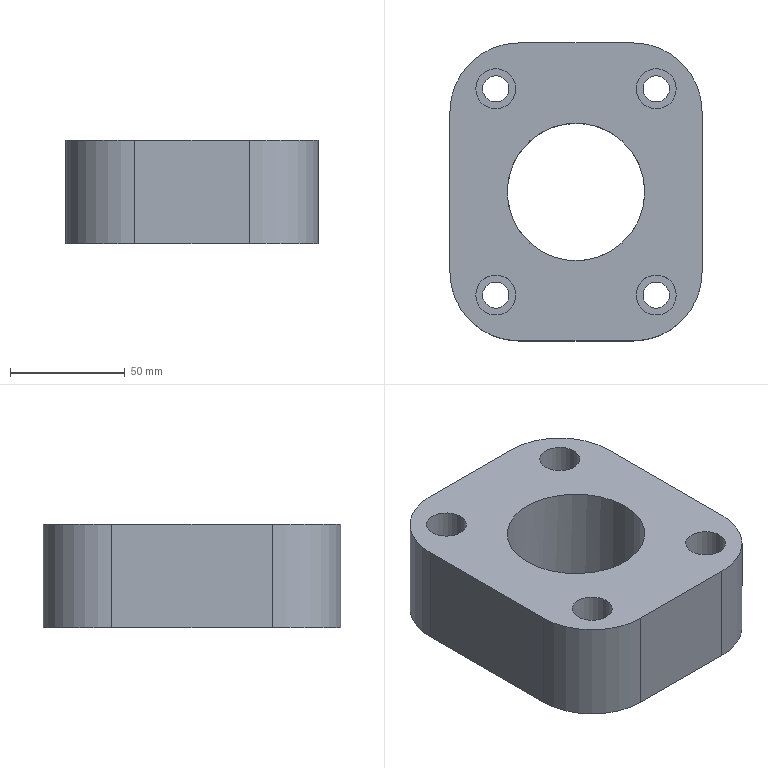Part | NX | features solid 2 | 1 solid | 23 faces | box 110 x 130 x 45 mm | volume 451871 mm3 | cylinder 13 | plane 10 | commonest cylinder face diameters 60 x5 11.5 x4 17.5 x4
STEP:
#1=CARTESIAN_POINT('',(-330.,55.,45.));
#2=VERTEX_POINT('',#1);
#3=CARTESIAN_POINT('',(-280.,55.,45.));
#4=VERTEX_POINT('',#3);
#5=CARTESIAN_POINT('',(-415.478,55.,45.));
#6=DIRECTION('',(-1.,0.,0.));
#7=VECTOR('',#6,1000.);
#8=LINE('',#5,#7);
#9=EDGE_CURVE('',#2,#4,#8,.F.);
#10=ORIENTED_EDGE('',*,*,#9,.T.);
#11=CARTESIAN_POINT('',(-250.,25.,45.));
#12=VERTEX_POINT('',#11);
#13=CARTESIAN_POINT('',(-280.,25.,45.));
#14=DIRECTION('',(0.,0.,1.));
#15=DIRECTION('',(1.,0.,0.));
#16=AXIS2_PLACEMENT_3D('',#13,#14,#15);
#17=CIRCLE('',#16,30.);
#18=EDGE_CURVE('',#4,#12,#17,.F.);
#19=ORIENTED_EDGE('',*,*,#18,.T.);
#20=CARTESIAN_POINT('',(-250.,-45.,45.));
#21=VERTEX_POINT('',#20);
#22=CARTESIAN_POINT('',(-250.,-10.,45.));
#23=DIRECTION('',(0.,-1.,0.));
#24=VECTOR('',#23,1000.);
#25=LINE('',#22,#24);
#26=EDGE_CURVE('',#21,#12,#25,.F.);
#27=ORIENTED_EDGE('',*,*,#26,.F.);
#28=CARTESIAN_POINT('',(-280.,-75.,45.));
#29=VERTEX_POINT('',#28);
#30=CARTESIAN_POINT('',(-280.,-45.,45.));
#31=DIRECTION('',(0.,0.,1.));
#32=DIRECTION('',(1.,0.,0.));
#33=AXIS2_PLACEMENT_3D('',#30,#31,#32);
#34=CIRCLE('',#33,30.);
#35=EDGE_CURVE('',#21,#29,#34,.F.);
#36=ORIENTED_EDGE('',*,*,#35,.T.);
#37=CARTESIAN_POINT('',(-330.,-75.,45.));
#38=VERTEX_POINT('',#37);
#39=CARTESIAN_POINT('',(-305.,-75.,45.));
#40=DIRECTION('',(-1.,0.,0.));
#41=VECTOR('',#40,1000.);
#42=LINE('',#39,#41);
#43=EDGE_CURVE('',#38,#29,#42,.F.);
#44=ORIENTED_EDGE('',*,*,#43,.F.);
#45=CARTESIAN_POINT('',(-360.,-45.,45.));
#46=VERTEX_POINT('',#45);
#47=CARTESIAN_POINT('',(-330.,-45.,45.));
#48=DIRECTION('',(0.,0.,1.));
#49=DIRECTION('',(1.,0.,0.));
#50=AXIS2_PLACEMENT_3D('',#47,#48,#49);
#51=CIRCLE('',#50,30.);
#52=EDGE_CURVE('',#38,#46,#51,.F.);
#53=ORIENTED_EDGE('',*,*,#52,.T.);
#54=CARTESIAN_POINT('',(-360.,25.,45.));
#55=VERTEX_POINT('',#54);
#56=CARTESIAN_POINT('',(-360.,-10.,45.));
#57=DIRECTION('',(0.,-1.,0.));
#58=VECTOR('',#57,1000.);
#59=LINE('',#56,#58);
#60=EDGE_CURVE('',#46,#55,#59,.F.);
#61=ORIENTED_EDGE('',*,*,#60,.T.);
#62=CARTESIAN_POINT('',(-330.,25.,45.));
#63=DIRECTION('',(0.,0.,1.));
#64=DIRECTION('',(1.,0.,0.));
#65=AXIS2_PLACEMENT_3D('',#62,#63,#64);
#66=CIRCLE('',#65,30.);
#67=EDGE_CURVE('',#55,#2,#66,.F.);
#68=ORIENTED_EDGE('',*,*,#67,.T.);
#69=EDGE_LOOP('',(#10,#19,#27,#36,#44,#53,#61,#68));
#70=FACE_BOUND('',#69,.T.);
#71=CARTESIAN_POINT('',(-334.25,35.,45.));
#72=VERTEX_POINT('',#71);
#73=CARTESIAN_POINT('',(-340.,35.,45.));
#74=DIRECTION('',(0.,0.,1.));
#75=DIRECTION('',(1.,0.,0.));
#76=AXIS2_PLACEMENT_3D('',#73,#74,#75);
#77=CIRCLE('',#76,5.75);
#78=EDGE_CURVE('',#72,#72,#77,.F.);
#79=ORIENTED_EDGE('',*,*,#78,.F.);
#80=EDGE_LOOP('',(#79));
#81=FACE_BOUND('',#80,.T.);
#82=CARTESIAN_POINT('',(-264.25,35.,45.));
#83=VERTEX_POINT('',#82);
#84=CARTESIAN_POINT('',(-270.,35.,45.));
#85=DIRECTION('',(0.,0.,1.));
#86=DIRECTION('',(1.,0.,0.));
#87=AXIS2_PLACEMENT_3D('',#84,#85,#86);
#88=CIRCLE('',#87,5.75);
#89=EDGE_CURVE('',#83,#83,#88,.F.);
#90=ORIENTED_EDGE('',*,*,#89,.F.);
#91=EDGE_LOOP('',(#90));
#92=FACE_BOUND('',#91,.T.);
#93=CARTESIAN_POINT('',(-334.25,-55.,45.));
#94=VERTEX_POINT('',#93);
#95=CARTESIAN_POINT('',(-340.,-55.,45.));
#96=DIRECTION('',(0.,0.,1.));
#97=DIRECTION('',(1.,0.,0.));
#98=AXIS2_PLACEMENT_3D('',#95,#96,#97);
#99=CIRCLE('',#98,5.75);
#100=EDGE_CURVE('',#94,#94,#99,.F.);
#101=ORIENTED_EDGE('',*,*,#100,.F.);
#102=EDGE_LOOP('',(#101));
#103=FACE_BOUND('',#102,.T.);
#104=CARTESIAN_POINT('',(-264.25,-55.,45.));
#105=VERTEX_POINT('',#104);
#106=CARTESIAN_POINT('',(-270.,-55.,45.));
#107=DIRECTION('',(0.,0.,1.));
#108=DIRECTION('',(1.,0.,0.));
#109=AXIS2_PLACEMENT_3D('',#106,#107,#108);
#110=CIRCLE('',#109,5.75);
#111=EDGE_CURVE('',#105,#105,#110,.F.);
#112=ORIENTED_EDGE('',*,*,#111,.F.);
#113=EDGE_LOOP('',(#112));
#114=FACE_BOUND('',#113,.T.);
#115=CARTESIAN_POINT('',(-275.,-10.,45.));
#116=VERTEX_POINT('',#115);
#117=CARTESIAN_POINT('',(-305.,-10.,45.));
#118=DIRECTION('',(0.,0.,1.));
#119=DIRECTION('',(1.,0.,0.));
#120=AXIS2_PLACEMENT_3D('',#117,#118,#119);
#121=CIRCLE('',#120,30.);
#122=EDGE_CURVE('',#116,#116,#121,.T.);
#123=ORIENTED_EDGE('',*,*,#122,.T.);
#124=EDGE_LOOP('',(#123));
#125=FACE_BOUND('',#124,.T.);
#126=CARTESIAN_POINT('',(-415.478,35.09,45.));
#127=DIRECTION('',(0.,0.,1.));
#128=DIRECTION('',(1.,0.,0.));
#129=AXIS2_PLACEMENT_3D('',#126,#127,#128);
#130=PLANE('',#129);
#131=ADVANCED_FACE('',(#70,#81,#92,#103,#114,#125),#130,.F.);
#132=CARTESIAN_POINT('',(-250.,-45.,90.));
#133=VERTEX_POINT('',#132);
#134=CARTESIAN_POINT('',(-250.,25.,90.));
#135=VERTEX_POINT('',#134);
#136=CARTESIAN_POINT('',(-250.,-10.,90.));
#137=DIRECTION('',(0.,-1.,0.));
#138=VECTOR('',#137,1000.);
#139=LINE('',#136,#138);
#140=EDGE_CURVE('',#133,#135,#139,.F.);
#141=ORIENTED_EDGE('',*,*,#140,.T.);
#142=CARTESIAN_POINT('',(-280.,55.,90.));
#143=VERTEX_POINT('',#142);
#144=CARTESIAN_POINT('',(-280.,25.,90.));
#145=DIRECTION('',(0.,0.,-1.));
#146=DIRECTION('',(-1.,0.,0.));
#147=AXIS2_PLACEMENT_3D('',#144,#145,#146);
#148=CIRCLE('',#147,30.);
#149=EDGE_CURVE('',#135,#143,#148,.F.);
#150=ORIENTED_EDGE('',*,*,#149,.T.);
#151=CARTESIAN_POINT('',(-330.,55.,90.));
#152=VERTEX_POINT('',#151);
#153=CARTESIAN_POINT('',(-305.,55.,90.));
#154=DIRECTION('',(1.,0.,0.));
#155=VECTOR('',#154,1000.);
#156=LINE('',#153,#155);
#157=EDGE_CURVE('',#152,#143,#156,.T.);
#158=ORIENTED_EDGE('',*,*,#157,.F.);
#159=CARTESIAN_POINT('',(-360.,25.,90.));
#160=VERTEX_POINT('',#159);
#161=CARTESIAN_POINT('',(-330.,25.,90.));
#162=DIRECTION('',(0.,0.,-1.));
#163=DIRECTION('',(-1.,0.,0.));
#164=AXIS2_PLACEMENT_3D('',#161,#162,#163);
#165=CIRCLE('',#164,30.);
#166=EDGE_CURVE('',#152,#160,#165,.F.);
#167=ORIENTED_EDGE('',*,*,#166,.T.);
#168=CARTESIAN_POINT('',(-360.,-45.,90.));
#169=VERTEX_POINT('',#168);
#170=CARTESIAN_POINT('',(-360.,-10.,90.));
#171=DIRECTION('',(0.,-1.,0.));
#172=VECTOR('',#171,1000.);
#173=LINE('',#170,#172);
#174=EDGE_CURVE('',#169,#160,#173,.F.);
#175=ORIENTED_EDGE('',*,*,#174,.F.);
#176=CARTESIAN_POINT('',(-330.,-75.,90.));
#177=VERTEX_POINT('',#176);
#178=CARTESIAN_POINT('',(-330.,-45.,90.));
#179=DIRECTION('',(0.,0.,-1.));
#180=DIRECTION('',(-1.,0.,0.));
#181=AXIS2_PLACEMENT_3D('',#178,#179,#180);
#182=CIRCLE('',#181,30.);
#183=EDGE_CURVE('',#169,#177,#182,.F.);
#184=ORIENTED_EDGE('',*,*,#183,.T.);
#185=CARTESIAN_POINT('',(-280.,-75.,90.));
#186=VERTEX_POINT('',#185);
#187=CARTESIAN_POINT('',(-305.,-75.,90.));
#188=DIRECTION('',(1.,0.,0.));
#189=VECTOR('',#188,1000.);
#190=LINE('',#187,#189);
#191=EDGE_CURVE('',#177,#186,#190,.T.);
#192=ORIENTED_EDGE('',*,*,#191,.T.);
#193=CARTESIAN_POINT('',(-280.,-45.,90.));
#194=DIRECTION('',(0.,0.,-1.));
#195=DIRECTION('',(-1.,0.,0.));
#196=AXIS2_PLACEMENT_3D('',#193,#194,#195);
#197=CIRCLE('',#196,30.);
#198=EDGE_CURVE('',#186,#133,#197,.F.);
#199=ORIENTED_EDGE('',*,*,#198,.T.);
#200=EDGE_LOOP('',(#141,#150,#158,#167,#175,#184,#192,#199));
#201=FACE_BOUND('',#200,.T.);
#202=CARTESIAN_POINT('',(-348.75,35.,90.));
#203=VERTEX_POINT('',#202);
#204=CARTESIAN_POINT('',(-340.,35.,90.));
#205=DIRECTION('',(0.,0.,-1.));
#206=DIRECTION('',(-1.,0.,0.));
#207=AXIS2_PLACEMENT_3D('',#204,#205,#206);
#208=CIRCLE('',#207,8.75);
#209=EDGE_CURVE('',#203,#203,#208,.T.);
#210=ORIENTED_EDGE('',*,*,#209,.T.);
#211=EDGE_LOOP('',(#210));
#212=FACE_BOUND('',#211,.T.);
#213=CARTESIAN_POINT('',(-278.75,35.,90.));
#214=VERTEX_POINT('',#213);
#215=CARTESIAN_POINT('',(-270.,35.,90.));
#216=DIRECTION('',(0.,0.,-1.));
#217=DIRECTION('',(-1.,0.,0.));
#218=AXIS2_PLACEMENT_3D('',#215,#216,#217);
#219=CIRCLE('',#218,8.75);
#220=EDGE_CURVE('',#214,#214,#219,.T.);
#221=ORIENTED_EDGE('',*,*,#220,.T.);
#222=EDGE_LOOP('',(#221));
#223=FACE_BOUND('',#222,.T.);
#224=CARTESIAN_POINT('',(-348.75,-55.,90.));
#225=VERTEX_POINT('',#224);
#226=CARTESIAN_POINT('',(-340.,-55.,90.));
#227=DIRECTION('',(0.,0.,-1.));
#228=DIRECTION('',(-1.,0.,0.));
#229=AXIS2_PLACEMENT_3D('',#226,#227,#228);
#230=CIRCLE('',#229,8.75);
#231=EDGE_CURVE('',#225,#225,#230,.T.);
#232=ORIENTED_EDGE('',*,*,#231,.T.);
#233=EDGE_LOOP('',(#232));
#234=FACE_BOUND('',#233,.T.);
#235=CARTESIAN_POINT('',(-278.75,-55.,90.));
#236=VERTEX_POINT('',#235);
#237=CARTESIAN_POINT('',(-270.,-55.,90.));
#238=DIRECTION('',(0.,0.,-1.));
#239=DIRECTION('',(-1.,0.,0.));
#240=AXIS2_PLACEMENT_3D('',#237,#238,#239);
#241=CIRCLE('',#240,8.75);
#242=EDGE_CURVE('',#236,#236,#241,.T.);
#243=ORIENTED_EDGE('',*,*,#242,.T.);
#244=EDGE_LOOP('',(#243));
#245=FACE_BOUND('',#244,.T.);
#246=CARTESIAN_POINT('',(-335.,-10.,90.));
#247=VERTEX_POINT('',#246);
#248=CARTESIAN_POINT('',(-305.,-10.,90.));
#249=DIRECTION('',(0.,0.,-1.));
#250=DIRECTION('',(-1.,0.,0.));
#251=AXIS2_PLACEMENT_3D('',#248,#249,#250);
#252=CIRCLE('',#251,30.);
#253=EDGE_CURVE('',#247,#247,#252,.T.);
#254=ORIENTED_EDGE('',*,*,#253,.T.);
#255=EDGE_LOOP('',(#254));
#256=FACE_BOUND('',#255,.T.);
#257=CARTESIAN_POINT('',(-305.,-10.,90.));
#258=DIRECTION('',(0.,0.,-1.));
#259=DIRECTION('',(0.,1.,0.));
#260=AXIS2_PLACEMENT_3D('',#257,#258,#259);
#261=PLANE('',#260);
#262=ADVANCED_FACE('',(#201,#212,#223,#234,#245,#256),#261,.F.);
#263=ORIENTED_EDGE('',*,*,#157,.T.);
#264=CARTESIAN_POINT('',(-280.,55.,60.));
#265=DIRECTION('',(0.,0.,1.));
#266=VECTOR('',#265,1000.);
#267=LINE('',#264,#266);
#268=EDGE_CURVE('',#143,#4,#267,.F.);
#269=ORIENTED_EDGE('',*,*,#268,.T.);
#270=ORIENTED_EDGE('',*,*,#9,.F.);
#271=CARTESIAN_POINT('',(-330.,55.,90.));
#272=DIRECTION('',(0.,0.,1.));
#273=VECTOR('',#272,1000.);
#274=LINE('',#271,#273);
#275=EDGE_CURVE('',#2,#152,#274,.T.);
#276=ORIENTED_EDGE('',*,*,#275,.T.);
#277=EDGE_LOOP('',(#263,#269,#270,#276));
#278=FACE_BOUND('',#277,.T.);
#279=CARTESIAN_POINT('',(-305.,55.,60.));
#280=DIRECTION('',(0.,1.,0.));
#281=DIRECTION('',(0.,0.,1.));
#282=AXIS2_PLACEMENT_3D('',#279,#280,#281);
#283=PLANE('',#282);
#284=ADVANCED_FACE('',(#278),#283,.T.);
#285=ORIENTED_EDGE('',*,*,#26,.T.);
#286=CARTESIAN_POINT('',(-250.,25.,60.));
#287=DIRECTION('',(0.,0.,1.));
#288=VECTOR('',#287,1000.);
#289=LINE('',#286,#288);
#290=EDGE_CURVE('',#12,#135,#289,.T.);
#291=ORIENTED_EDGE('',*,*,#290,.T.);
#292=ORIENTED_EDGE('',*,*,#140,.F.);
#293=CARTESIAN_POINT('',(-250.,-45.,60.));
#294=DIRECTION('',(0.,0.,1.));
#295=VECTOR('',#294,1000.);
#296=LINE('',#293,#295);
#297=EDGE_CURVE('',#133,#21,#296,.F.);
#298=ORIENTED_EDGE('',*,*,#297,.T.);
#299=EDGE_LOOP('',(#285,#291,#292,#298));
#300=FACE_BOUND('',#299,.T.);
#301=CARTESIAN_POINT('',(-250.,-10.,60.));
#302=DIRECTION('',(1.,0.,0.));
#303=DIRECTION('',(0.,0.,-1.));
#304=AXIS2_PLACEMENT_3D('',#301,#302,#303);
#305=PLANE('',#304);
#306=ADVANCED_FACE('',(#300),#305,.T.);
#307=ORIENTED_EDGE('',*,*,#174,.T.);
#308=CARTESIAN_POINT('',(-360.,25.,60.));
#309=DIRECTION('',(0.,0.,1.));
#310=VECTOR('',#309,1000.);
#311=LINE('',#308,#310);
#312=EDGE_CURVE('',#160,#55,#311,.F.);
#313=ORIENTED_EDGE('',*,*,#312,.T.);
#314=ORIENTED_EDGE('',*,*,#60,.F.);
#315=CARTESIAN_POINT('',(-360.,-45.,90.));
#316=DIRECTION('',(0.,0.,1.));
#317=VECTOR('',#316,1000.);
#318=LINE('',#315,#317);
#319=EDGE_CURVE('',#46,#169,#318,.T.);
#320=ORIENTED_EDGE('',*,*,#319,.T.);
#321=EDGE_LOOP('',(#307,#313,#314,#320));
#322=FACE_BOUND('',#321,.T.);
#323=CARTESIAN_POINT('',(-360.,-10.,60.));
#324=DIRECTION('',(1.,0.,0.));
#325=DIRECTION('',(0.,0.,-1.));
#326=AXIS2_PLACEMENT_3D('',#323,#324,#325);
#327=PLANE('',#326);
#328=ADVANCED_FACE('',(#322),#327,.F.);
#329=ORIENTED_EDGE('',*,*,#191,.F.);
#330=CARTESIAN_POINT('',(-330.,-75.,60.));
#331=DIRECTION('',(0.,0.,1.));
#332=VECTOR('',#331,1000.);
#333=LINE('',#330,#332);
#334=EDGE_CURVE('',#177,#38,#333,.F.);
#335=ORIENTED_EDGE('',*,*,#334,.T.);
#336=ORIENTED_EDGE('',*,*,#43,.T.);
#337=CARTESIAN_POINT('',(-280.,-75.,60.));
#338=DIRECTION('',(0.,0.,1.));
#339=VECTOR('',#338,1000.);
#340=LINE('',#337,#339);
#341=EDGE_CURVE('',#29,#186,#340,.T.);
#342=ORIENTED_EDGE('',*,*,#341,.T.);
#343=EDGE_LOOP('',(#329,#335,#336,#342));
#344=FACE_BOUND('',#343,.T.);
#345=CARTESIAN_POINT('',(-305.,-75.,60.));
#346=DIRECTION('',(0.,-1.,0.));
#347=DIRECTION('',(0.,0.,1.));
#348=AXIS2_PLACEMENT_3D('',#345,#346,#347);
#349=PLANE('',#348);
#350=ADVANCED_FACE('',(#344),#349,.T.);
#351=ORIENTED_EDGE('',*,*,#18,.F.);
#352=ORIENTED_EDGE('',*,*,#268,.F.);
#353=ORIENTED_EDGE('',*,*,#149,.F.);
#354=ORIENTED_EDGE('',*,*,#290,.F.);
#355=EDGE_LOOP('',(#351,#352,#353,#354));
#356=FACE_BOUND('',#355,.T.);
#357=CARTESIAN_POINT('',(-280.,25.,60.));
#358=DIRECTION('',(0.,0.,1.));
#359=DIRECTION('',(1.,0.,0.));
#360=AXIS2_PLACEMENT_3D('',#357,#358,#359);
#361=CYLINDRICAL_SURFACE('',#360,30.);
#362=ADVANCED_FACE('',(#356),#361,.T.);
#363=ORIENTED_EDGE('',*,*,#67,.F.);
#364=ORIENTED_EDGE('',*,*,#312,.F.);
#365=ORIENTED_EDGE('',*,*,#166,.F.);
#366=ORIENTED_EDGE('',*,*,#275,.F.);
#367=EDGE_LOOP('',(#363,#364,#365,#366));
#368=FACE_BOUND('',#367,.T.);
#369=CARTESIAN_POINT('',(-330.,25.,60.));
#370=DIRECTION('',(0.,0.,-1.));
#371=DIRECTION('',(-1.,0.,0.));
#372=AXIS2_PLACEMENT_3D('',#369,#370,#371);
#373=CYLINDRICAL_SURFACE('',#372,30.);
#374=ADVANCED_FACE('',(#368),#373,.T.);
#375=ORIENTED_EDGE('',*,*,#52,.F.);
#376=ORIENTED_EDGE('',*,*,#334,.F.);
#377=ORIENTED_EDGE('',*,*,#183,.F.);
#378=ORIENTED_EDGE('',*,*,#319,.F.);
#379=EDGE_LOOP('',(#375,#376,#377,#378));
#380=FACE_BOUND('',#379,.T.);
#381=CARTESIAN_POINT('',(-330.,-45.,60.));
#382=DIRECTION('',(0.,0.,-1.));
#383=DIRECTION('',(-1.,0.,0.));
#384=AXIS2_PLACEMENT_3D('',#381,#382,#383);
#385=CYLINDRICAL_SURFACE('',#384,30.);
#386=ADVANCED_FACE('',(#380),#385,.T.);
#387=ORIENTED_EDGE('',*,*,#35,.F.);
#388=ORIENTED_EDGE('',*,*,#297,.F.);
#389=ORIENTED_EDGE('',*,*,#198,.F.);
#390=ORIENTED_EDGE('',*,*,#341,.F.);
#391=EDGE_LOOP('',(#387,#388,#389,#390));
#392=FACE_BOUND('',#391,.T.);
#393=CARTESIAN_POINT('',(-280.,-45.,60.));
#394=DIRECTION('',(0.,0.,1.));
#395=DIRECTION('',(1.,0.,0.));
#396=AXIS2_PLACEMENT_3D('',#393,#394,#395);
#397=CYLINDRICAL_SURFACE('',#396,30.);
#398=ADVANCED_FACE('',(#392),#397,.T.);
#399=ORIENTED_EDGE('',*,*,#78,.T.);
#400=EDGE_LOOP('',(#399));
#401=FACE_BOUND('',#400,.T.);
#402=CARTESIAN_POINT('',(-345.75,35.,70.));
#403=VERTEX_POINT('',#402);
#404=CARTESIAN_POINT('',(-340.,35.,70.));
#405=DIRECTION('',(0.,0.,-1.));
#406=DIRECTION('',(-1.,0.,0.));
#407=AXIS2_PLACEMENT_3D('',#404,#405,#406);
#408=CIRCLE('',#407,5.75);
#409=EDGE_CURVE('',#403,#403,#408,.T.);
#410=ORIENTED_EDGE('',*,*,#409,.F.);
#411=EDGE_LOOP('',(#410));
#412=FACE_BOUND('',#411,.T.);
#413=CARTESIAN_POINT('',(-340.,35.,40.));
#414=DIRECTION('',(0.,0.,-1.));
#415=DIRECTION('',(-1.,0.,0.));
#416=AXIS2_PLACEMENT_3D('',#413,#414,#415);
#417=CYLINDRICAL_SURFACE('',#416,5.75);
#418=ADVANCED_FACE('',(#401,#412),#417,.F.);
#419=ORIENTED_EDGE('',*,*,#409,.T.);
#420=EDGE_LOOP('',(#419));
#421=FACE_BOUND('',#420,.T.);
#422=CARTESIAN_POINT('',(-348.75,35.,70.));
#423=VERTEX_POINT('',#422);
#424=CARTESIAN_POINT('',(-340.,35.,70.));
#425=DIRECTION('',(0.,0.,-1.));
#426=DIRECTION('',(-1.,0.,0.));
#427=AXIS2_PLACEMENT_3D('',#424,#425,#426);
#428=CIRCLE('',#427,8.75);
#429=EDGE_CURVE('',#423,#423,#428,.T.);
#430=ORIENTED_EDGE('',*,*,#429,.F.);
#431=EDGE_LOOP('',(#430));
#432=FACE_BOUND('',#431,.T.);
#433=CARTESIAN_POINT('',(-340.,35.,70.));
#434=DIRECTION('',(0.,0.,-1.));
#435=DIRECTION('',(-1.,0.,0.));
#436=AXIS2_PLACEMENT_3D('',#433,#434,#435);
#437=PLANE('',#436);
#438=ADVANCED_FACE('',(#421,#432),#437,.F.);
#439=ORIENTED_EDGE('',*,*,#429,.T.);
#440=EDGE_LOOP('',(#439));
#441=FACE_BOUND('',#440,.T.);
#442=ORIENTED_EDGE('',*,*,#209,.F.);
#443=EDGE_LOOP('',(#442));
#444=FACE_BOUND('',#443,.T.);
#445=CARTESIAN_POINT('',(-340.,35.,90.));
#446=DIRECTION('',(0.,0.,-1.));
#447=DIRECTION('',(-1.,0.,0.));
#448=AXIS2_PLACEMENT_3D('',#445,#446,#447);
#449=CYLINDRICAL_SURFACE('',#448,8.75);
#450=ADVANCED_FACE('',(#441,#444),#449,.F.);
#451=ORIENTED_EDGE('',*,*,#89,.T.);
#452=EDGE_LOOP('',(#451));
#453=FACE_BOUND('',#452,.T.);
#454=CARTESIAN_POINT('',(-275.75,35.,70.));
#455=VERTEX_POINT('',#454);
#456=CARTESIAN_POINT('',(-270.,35.,70.));
#457=DIRECTION('',(0.,0.,-1.));
#458=DIRECTION('',(-1.,0.,0.));
#459=AXIS2_PLACEMENT_3D('',#456,#457,#458);
#460=CIRCLE('',#459,5.75);
#461=EDGE_CURVE('',#455,#455,#460,.T.);
#462=ORIENTED_EDGE('',*,*,#461,.F.);
#463=EDGE_LOOP('',(#462));
#464=FACE_BOUND('',#463,.T.);
#465=CARTESIAN_POINT('',(-270.,35.,40.));
#466=DIRECTION('',(0.,0.,-1.));
#467=DIRECTION('',(-1.,0.,0.));
#468=AXIS2_PLACEMENT_3D('',#465,#466,#467);
#469=CYLINDRICAL_SURFACE('',#468,5.75);
#470=ADVANCED_FACE('',(#453,#464),#469,.F.);
#471=ORIENTED_EDGE('',*,*,#461,.T.);
#472=EDGE_LOOP('',(#471));
#473=FACE_BOUND('',#472,.T.);
#474=CARTESIAN_POINT('',(-278.75,35.,70.));
#475=VERTEX_POINT('',#474);
#476=CARTESIAN_POINT('',(-270.,35.,70.));
#477=DIRECTION('',(0.,0.,-1.));
#478=DIRECTION('',(-1.,0.,0.));
#479=AXIS2_PLACEMENT_3D('',#476,#477,#478);
#480=CIRCLE('',#479,8.75);
#481=EDGE_CURVE('',#475,#475,#480,.T.);
#482=ORIENTED_EDGE('',*,*,#481,.F.);
#483=EDGE_LOOP('',(#482));
#484=FACE_BOUND('',#483,.T.);
#485=CARTESIAN_POINT('',(-270.,35.,70.));
#486=DIRECTION('',(0.,0.,-1.));
#487=DIRECTION('',(-1.,0.,0.));
#488=AXIS2_PLACEMENT_3D('',#485,#486,#487);
#489=PLANE('',#488);
#490=ADVANCED_FACE('',(#473,#484),#489,.F.);
#491=ORIENTED_EDGE('',*,*,#481,.T.);
#492=EDGE_LOOP('',(#491));
#493=FACE_BOUND('',#492,.T.);
#494=ORIENTED_EDGE('',*,*,#220,.F.);
#495=EDGE_LOOP('',(#494));
#496=FACE_BOUND('',#495,.T.);
#497=CARTESIAN_POINT('',(-270.,35.,90.));
#498=DIRECTION('',(0.,0.,-1.));
#499=DIRECTION('',(-1.,0.,0.));
#500=AXIS2_PLACEMENT_3D('',#497,#498,#499);
#501=CYLINDRICAL_SURFACE('',#500,8.75);
#502=ADVANCED_FACE('',(#493,#496),#501,.F.);
#503=ORIENTED_EDGE('',*,*,#100,.T.);
#504=EDGE_LOOP('',(#503));
#505=FACE_BOUND('',#504,.T.);
#506=CARTESIAN_POINT('',(-345.75,-55.,70.));
#507=VERTEX_POINT('',#506);
#508=CARTESIAN_POINT('',(-340.,-55.,70.));
#509=DIRECTION('',(0.,0.,-1.));
#510=DIRECTION('',(-1.,0.,0.));
#511=AXIS2_PLACEMENT_3D('',#508,#509,#510);
#512=CIRCLE('',#511,5.75);
#513=EDGE_CURVE('',#507,#507,#512,.T.);
#514=ORIENTED_EDGE('',*,*,#513,.F.);
#515=EDGE_LOOP('',(#514));
#516=FACE_BOUND('',#515,.T.);
#517=CARTESIAN_POINT('',(-340.,-55.,40.));
#518=DIRECTION('',(0.,0.,-1.));
#519=DIRECTION('',(-1.,0.,0.));
#520=AXIS2_PLACEMENT_3D('',#517,#518,#519);
#521=CYLINDRICAL_SURFACE('',#520,5.75);
#522=ADVANCED_FACE('',(#505,#516),#521,.F.);
#523=ORIENTED_EDGE('',*,*,#513,.T.);
#524=EDGE_LOOP('',(#523));
#525=FACE_BOUND('',#524,.T.);
#526=CARTESIAN_POINT('',(-348.75,-55.,70.));
#527=VERTEX_POINT('',#526);
#528=CARTESIAN_POINT('',(-340.,-55.,70.));
#529=DIRECTION('',(0.,0.,-1.));
#530=DIRECTION('',(-1.,0.,0.));
#531=AXIS2_PLACEMENT_3D('',#528,#529,#530);
#532=CIRCLE('',#531,8.75);
#533=EDGE_CURVE('',#527,#527,#532,.T.);
#534=ORIENTED_EDGE('',*,*,#533,.F.);
#535=EDGE_LOOP('',(#534));
#536=FACE_BOUND('',#535,.T.);
#537=CARTESIAN_POINT('',(-340.,-55.,70.));
#538=DIRECTION('',(0.,0.,-1.));
#539=DIRECTION('',(-1.,0.,0.));
#540=AXIS2_PLACEMENT_3D('',#537,#538,#539);
#541=PLANE('',#540);
#542=ADVANCED_FACE('',(#525,#536),#541,.F.);
#543=ORIENTED_EDGE('',*,*,#533,.T.);
#544=EDGE_LOOP('',(#543));
#545=FACE_BOUND('',#544,.T.);
#546=ORIENTED_EDGE('',*,*,#231,.F.);
#547=EDGE_LOOP('',(#546));
#548=FACE_BOUND('',#547,.T.);
#549=CARTESIAN_POINT('',(-340.,-55.,90.));
#550=DIRECTION('',(0.,0.,-1.));
#551=DIRECTION('',(-1.,0.,0.));
#552=AXIS2_PLACEMENT_3D('',#549,#550,#551);
#553=CYLINDRICAL_SURFACE('',#552,8.75);
#554=ADVANCED_FACE('',(#545,#548),#553,.F.);
#555=ORIENTED_EDGE('',*,*,#111,.T.);
#556=EDGE_LOOP('',(#555));
#557=FACE_BOUND('',#556,.T.);
#558=CARTESIAN_POINT('',(-275.75,-55.,70.));
#559=VERTEX_POINT('',#558);
#560=CARTESIAN_POINT('',(-270.,-55.,70.));
#561=DIRECTION('',(0.,0.,-1.));
#562=DIRECTION('',(-1.,0.,0.));
#563=AXIS2_PLACEMENT_3D('',#560,#561,#562);
#564=CIRCLE('',#563,5.75);
#565=EDGE_CURVE('',#559,#559,#564,.T.);
#566=ORIENTED_EDGE('',*,*,#565,.F.);
#567=EDGE_LOOP('',(#566));
#568=FACE_BOUND('',#567,.T.);
#569=CARTESIAN_POINT('',(-270.,-55.,40.));
#570=DIRECTION('',(0.,0.,-1.));
#571=DIRECTION('',(-1.,0.,0.));
#572=AXIS2_PLACEMENT_3D('',#569,#570,#571);
#573=CYLINDRICAL_SURFACE('',#572,5.75);
#574=ADVANCED_FACE('',(#557,#568),#573,.F.);
#575=ORIENTED_EDGE('',*,*,#565,.T.);
#576=EDGE_LOOP('',(#575));
#577=FACE_BOUND('',#576,.T.);
#578=CARTESIAN_POINT('',(-278.75,-55.,70.));
#579=VERTEX_POINT('',#578);
#580=CARTESIAN_POINT('',(-270.,-55.,70.));
#581=DIRECTION('',(0.,0.,-1.));
#582=DIRECTION('',(-1.,0.,0.));
#583=AXIS2_PLACEMENT_3D('',#580,#581,#582);
#584=CIRCLE('',#583,8.75);
#585=EDGE_CURVE('',#579,#579,#584,.T.);
#586=ORIENTED_EDGE('',*,*,#585,.F.);
#587=EDGE_LOOP('',(#586));
#588=FACE_BOUND('',#587,.T.);
#589=CARTESIAN_POINT('',(-270.,-55.,70.));
#590=DIRECTION('',(0.,0.,-1.));
#591=DIRECTION('',(-1.,0.,0.));
#592=AXIS2_PLACEMENT_3D('',#589,#590,#591);
#593=PLANE('',#592);
#594=ADVANCED_FACE('',(#577,#588),#593,.F.);
#595=ORIENTED_EDGE('',*,*,#585,.T.);
#596=EDGE_LOOP('',(#595));
#597=FACE_BOUND('',#596,.T.);
#598=ORIENTED_EDGE('',*,*,#242,.F.);
#599=EDGE_LOOP('',(#598));
#600=FACE_BOUND('',#599,.T.);
#601=CARTESIAN_POINT('',(-270.,-55.,90.));
#602=DIRECTION('',(0.,0.,-1.));
#603=DIRECTION('',(-1.,0.,0.));
#604=AXIS2_PLACEMENT_3D('',#601,#602,#603);
#605=CYLINDRICAL_SURFACE('',#604,8.75);
#606=ADVANCED_FACE('',(#597,#600),#605,.F.);
#607=ORIENTED_EDGE('',*,*,#122,.F.);
#608=EDGE_LOOP('',(#607));
#609=FACE_BOUND('',#608,.T.);
#610=ORIENTED_EDGE('',*,*,#253,.F.);
#611=EDGE_LOOP('',(#610));
#612=FACE_BOUND('',#611,.T.);
#613=CARTESIAN_POINT('',(-305.,-10.,30.));
#614=DIRECTION('',(0.,0.,1.));
#615=DIRECTION('',(1.,0.,0.));
#616=AXIS2_PLACEMENT_3D('',#613,#614,#615);
#617=CYLINDRICAL_SURFACE('',#616,30.);
#618=ADVANCED_FACE('',(#609,#612),#617,.F.);
#619=CLOSED_SHELL('',(#131,#262,#284,#306,#328,#350,#362,#374,#386,#398,#418,#438,#450,#470,#490,#502,#522,#542,#554,#574,#594,#606,#618));
#620=MANIFOLD_SOLID_BREP('',#619);
#621=(LENGTH_UNIT()NAMED_UNIT(*)SI_UNIT(.MILLI.,.METRE.));
#622=UNCERTAINTY_MEASURE_WITH_UNIT(LENGTH_MEASURE(0.00001),#621,'','');
#623=(NAMED_UNIT(*)PLANE_ANGLE_UNIT()SI_UNIT($,.RADIAN.));
#624=(NAMED_UNIT(*)SI_UNIT($,.STERADIAN.)SOLID_ANGLE_UNIT());
#625=(GEOMETRIC_REPRESENTATION_CONTEXT(3)GLOBAL_UNCERTAINTY_ASSIGNED_CONTEXT((#622))GLOBAL_UNIT_ASSIGNED_CONTEXT((#621,#623,#624))REPRESENTATION_CONTEXT('',''));
#626=ADVANCED_BREP_SHAPE_REPRESENTATION('',(#620),#625);